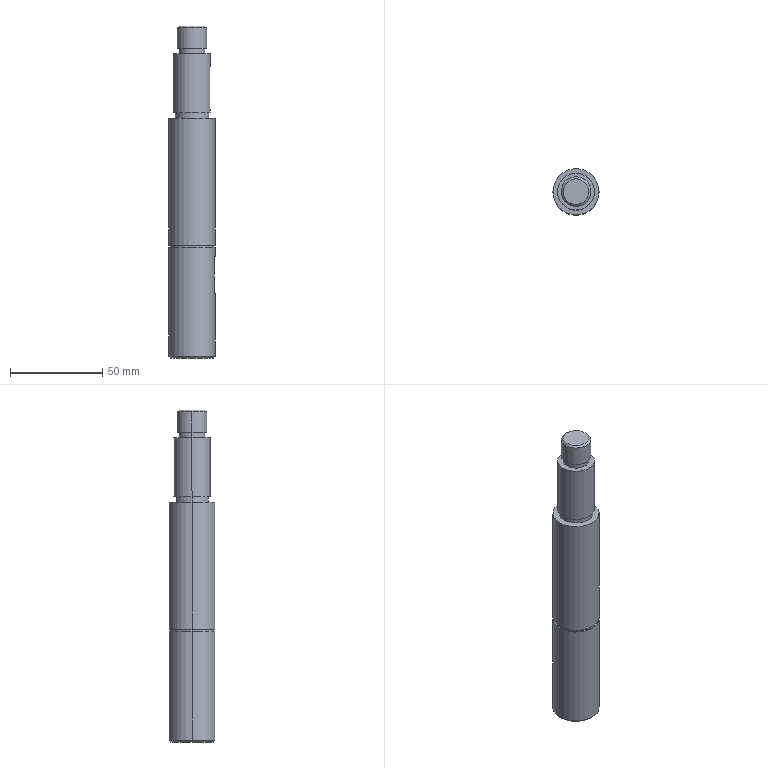Part | SolidWorks | features Chamfer 1, ICE 1, RefSurface 1, Revolution 1, ThickenCut 1 | 1 solid | 35 faces | box 25 x 25 x 180 mm | volume 76361 mm3 | cylinder 18 | plane 13 | cone 4 | commonest cylinder face diameters 25 x4 6 x3 14 x2 16 x2 18 x2 20 x2
STEP:
#1=CARTESIAN_POINT('',(-11.5,0.,0.));
#2=VERTEX_POINT('',#1);
#3=CARTESIAN_POINT('',(11.5,0.,0.));
#4=VERTEX_POINT('',#3);
#5=CARTESIAN_POINT('',(0.,0.,0.));
#6=DIRECTION('',(0.,0.,-1.));
#7=DIRECTION('',(-1.,0.,0.));
#8=AXIS2_PLACEMENT_3D('',#5,#6,#7);
#9=CIRCLE('',#8,11.5);
#10=EDGE_CURVE('',#2,#4,#9,.T.);
#11=ORIENTED_EDGE('',*,*,#10,.F.);
#12=CARTESIAN_POINT('',(-12.5,0.,1.));
#13=VERTEX_POINT('',#12);
#14=CARTESIAN_POINT('',(-11.5,0.,0.));
#15=DIRECTION('',(-0.7071,0.,0.7071));
#16=VECTOR('',#15,1000.);
#17=LINE('',#14,#16);
#18=EDGE_CURVE('',#2,#13,#17,.T.);
#19=ORIENTED_EDGE('',*,*,#18,.T.);
#20=CARTESIAN_POINT('',(12.5,0.,1.));
#21=VERTEX_POINT('',#20);
#22=CARTESIAN_POINT('',(0.,0.,1.));
#23=DIRECTION('',(0.,0.,1.));
#24=DIRECTION('',(-1.,0.,0.));
#25=AXIS2_PLACEMENT_3D('',#22,#23,#24);
#26=CIRCLE('',#25,12.5);
#27=EDGE_CURVE('',#21,#13,#26,.T.);
#28=ORIENTED_EDGE('',*,*,#27,.F.);
#29=CARTESIAN_POINT('',(11.5,0.,0.));
#30=DIRECTION('',(0.7071,0.,0.7071));
#31=VECTOR('',#30,1000.);
#32=LINE('',#29,#31);
#33=EDGE_CURVE('',#4,#21,#32,.T.);
#34=ORIENTED_EDGE('',*,*,#33,.F.);
#35=EDGE_LOOP('',(#11,#19,#28,#34));
#36=FACE_OUTER_BOUND('',#35,.T.);
#37=CARTESIAN_POINT('',(0.,0.,0.));
#38=DIRECTION('',(0.,0.,1.));
#39=DIRECTION('',(1.,0.,0.));
#40=AXIS2_PLACEMENT_3D('',#37,#38,#39);
#41=CONICAL_SURFACE('',#40,11.5,0.7854);
#42=ADVANCED_FACE('',(#36),#41,.T.);
#43=CARTESIAN_POINT('',(7.,0.,180.));
#44=VERTEX_POINT('',#43);
#45=CARTESIAN_POINT('',(-7.,0.,180.));
#46=VERTEX_POINT('',#45);
#47=CARTESIAN_POINT('',(0.,0.,180.));
#48=DIRECTION('',(0.,0.,1.));
#49=DIRECTION('',(1.,0.,0.));
#50=AXIS2_PLACEMENT_3D('',#47,#48,#49);
#51=CIRCLE('',#50,7.);
#52=EDGE_CURVE('',#44,#46,#51,.T.);
#53=ORIENTED_EDGE('',*,*,#52,.F.);
#54=CARTESIAN_POINT('',(8.,0.,179.));
#55=VERTEX_POINT('',#54);
#56=CARTESIAN_POINT('',(8.,0.,179.));
#57=DIRECTION('',(0.7071,0.,-0.7071));
#58=VECTOR('',#57,1000.);
#59=LINE('',#56,#58);
#60=EDGE_CURVE('',#44,#55,#59,.T.);
#61=ORIENTED_EDGE('',*,*,#60,.T.);
#62=CARTESIAN_POINT('',(-8.,0.,179.));
#63=VERTEX_POINT('',#62);
#64=CARTESIAN_POINT('',(0.,0.,179.));
#65=DIRECTION('',(0.,0.,-1.));
#66=DIRECTION('',(1.,0.,0.));
#67=AXIS2_PLACEMENT_3D('',#64,#65,#66);
#68=CIRCLE('',#67,8.);
#69=EDGE_CURVE('',#63,#55,#68,.T.);
#70=ORIENTED_EDGE('',*,*,#69,.F.);
#71=CARTESIAN_POINT('',(-8.,0.,179.));
#72=DIRECTION('',(-0.7071,0.,-0.7071));
#73=VECTOR('',#72,1000.);
#74=LINE('',#71,#73);
#75=EDGE_CURVE('',#46,#63,#74,.T.);
#76=ORIENTED_EDGE('',*,*,#75,.F.);
#77=EDGE_LOOP('',(#53,#61,#70,#76));
#78=FACE_OUTER_BOUND('',#77,.T.);
#79=CARTESIAN_POINT('',(0.,0.,179.));
#80=DIRECTION('',(0.,0.,-1.));
#81=DIRECTION('',(-1.,0.,0.));
#82=AXIS2_PLACEMENT_3D('',#79,#80,#81);
#83=CONICAL_SURFACE('',#82,8.,0.7854);
#84=ADVANCED_FACE('',(#78),#83,.T.);
#85=CARTESIAN_POINT('',(9.539,3.,156.));
#86=VERTEX_POINT('',#85);
#87=CARTESIAN_POINT('',(10.,0.,159.));
#88=VERTEX_POINT('',#87);
#89=CARTESIAN_POINT('',(9.539,3.,156.));
#90=CARTESIAN_POINT('',(9.539,3.,156.2));
#91=CARTESIAN_POINT('',(9.546,2.98,156.395));
#92=CARTESIAN_POINT('',(9.569,2.903,156.781));
#93=CARTESIAN_POINT('',(9.587,2.845,156.972));
#94=CARTESIAN_POINT('',(9.631,2.694,157.335));
#95=CARTESIAN_POINT('',(9.656,2.602,157.506));
#96=CARTESIAN_POINT('',(9.712,2.384,157.832));
#97=CARTESIAN_POINT('',(9.743,2.258,157.985));
#98=CARTESIAN_POINT('',(9.832,1.845,158.397));
#99=CARTESIAN_POINT('',(9.892,1.512,158.62));
#100=CARTESIAN_POINT('',(9.954,0.971,158.845));
#101=CARTESIAN_POINT('',(9.971,0.7806,158.903));
#102=CARTESIAN_POINT('',(9.994,0.3926,158.981));
#103=CARTESIAN_POINT('',(10.,0.197,159.));
#104=CARTESIAN_POINT('',(10.,0.,159.));
#105=B_SPLINE_CURVE_WITH_KNOTS('',3,(#89,#90,#91,#92,#93,#94,#95,#96,#97,#98,#99,#100,#101,#102,#103,#104),.UNSPECIFIED.,.F.,.F.,(4,2,2,2,2,2,2,4),(0.,0.0005898,0.00118,0.001769,0.002359,0.003539,0.004128,0.004718),.UNSPECIFIED.);
#106=EDGE_CURVE('',#86,#88,#105,.T.);
#107=ORIENTED_EDGE('',*,*,#106,.T.);
#108=CARTESIAN_POINT('',(6.5,0.,159.));
#109=VERTEX_POINT('',#108);
#110=CARTESIAN_POINT('',(12.5,0.,159.));
#111=DIRECTION('',(-1.,0.,0.));
#112=VECTOR('',#111,1000.);
#113=LINE('',#110,#112);
#114=EDGE_CURVE('',#88,#109,#113,.T.);
#115=ORIENTED_EDGE('',*,*,#114,.T.);
#116=CARTESIAN_POINT('',(6.5,3.,156.));
#117=VERTEX_POINT('',#116);
#118=CARTESIAN_POINT('',(6.5,0.,156.));
#119=DIRECTION('',(-1.,0.,0.));
#120=DIRECTION('',(0.,0.,1.));
#121=AXIS2_PLACEMENT_3D('',#118,#119,#120);
#122=CIRCLE('',#121,3.);
#123=EDGE_CURVE('',#109,#117,#122,.T.);
#124=ORIENTED_EDGE('',*,*,#123,.T.);
#125=CARTESIAN_POINT('',(12.5,3.,156.));
#126=DIRECTION('',(-1.,0.,0.));
#127=VECTOR('',#126,1000.);
#128=LINE('',#125,#127);
#129=EDGE_CURVE('',#86,#117,#128,.T.);
#130=ORIENTED_EDGE('',*,*,#129,.F.);
#131=EDGE_LOOP('',(#107,#115,#124,#130));
#132=FACE_OUTER_BOUND('',#131,.T.);
#133=CARTESIAN_POINT('',(12.5,0.,156.));
#134=DIRECTION('',(-1.,0.,0.));
#135=DIRECTION('',(0.,0.,1.));
#136=AXIS2_PLACEMENT_3D('',#133,#134,#135);
#137=CYLINDRICAL_SURFACE('',#136,3.);
#138=ADVANCED_FACE('',(#132),#137,.F.);
#139=CARTESIAN_POINT('',(-7.,0.,168.));
#140=VERTEX_POINT('',#139);
#141=CARTESIAN_POINT('',(7.,0.,168.));
#142=VERTEX_POINT('',#141);
#143=CARTESIAN_POINT('',(0.,0.,168.));
#144=DIRECTION('',(0.,0.,-1.));
#145=DIRECTION('',(-1.,0.,0.));
#146=AXIS2_PLACEMENT_3D('',#143,#144,#145);
#147=CIRCLE('',#146,7.);
#148=EDGE_CURVE('',#140,#142,#147,.T.);
#149=ORIENTED_EDGE('',*,*,#148,.T.);
#150=CARTESIAN_POINT('',(7.,0.,165.));
#151=VERTEX_POINT('',#150);
#152=CARTESIAN_POINT('',(7.,0.,180.));
#153=DIRECTION('',(0.,0.,-1.));
#154=VECTOR('',#153,1000.);
#155=LINE('',#152,#154);
#156=EDGE_CURVE('',#142,#151,#155,.T.);
#157=ORIENTED_EDGE('',*,*,#156,.T.);
#158=CARTESIAN_POINT('',(-7.,0.,165.));
#159=VERTEX_POINT('',#158);
#160=CARTESIAN_POINT('',(0.,0.,165.));
#161=DIRECTION('',(0.,0.,-1.));
#162=DIRECTION('',(-1.,0.,0.));
#163=AXIS2_PLACEMENT_3D('',#160,#161,#162);
#164=CIRCLE('',#163,7.);
#165=EDGE_CURVE('',#159,#151,#164,.T.);
#166=ORIENTED_EDGE('',*,*,#165,.F.);
#167=CARTESIAN_POINT('',(-7.,0.,180.));
#168=DIRECTION('',(0.,0.,-1.));
#169=VECTOR('',#168,1000.);
#170=LINE('',#167,#169);
#171=EDGE_CURVE('',#140,#159,#170,.T.);
#172=ORIENTED_EDGE('',*,*,#171,.F.);
#173=EDGE_LOOP('',(#149,#157,#166,#172));
#174=FACE_OUTER_BOUND('',#173,.T.);
#175=CARTESIAN_POINT('',(0.,0.,180.));
#176=DIRECTION('',(0.,0.,-1.));
#177=DIRECTION('',(-1.,0.,0.));
#178=AXIS2_PLACEMENT_3D('',#175,#176,#177);
#179=CYLINDRICAL_SURFACE('',#178,7.);
#180=ADVANCED_FACE('',(#174),#179,.T.);
#181=CARTESIAN_POINT('',(-10.,0.,165.));
#182=VERTEX_POINT('',#181);
#183=CARTESIAN_POINT('',(10.,0.,165.));
#184=VERTEX_POINT('',#183);
#185=CARTESIAN_POINT('',(0.,0.,165.));
#186=DIRECTION('',(0.,0.,-1.));
#187=DIRECTION('',(-1.,0.,0.));
#188=AXIS2_PLACEMENT_3D('',#185,#186,#187);
#189=CIRCLE('',#188,10.);
#190=EDGE_CURVE('',#182,#184,#189,.T.);
#191=ORIENTED_EDGE('',*,*,#190,.T.);
#192=CARTESIAN_POINT('',(10.,0.,180.));
#193=DIRECTION('',(0.,0.,-1.));
#194=VECTOR('',#193,1000.);
#195=LINE('',#192,#194);
#196=EDGE_CURVE('',#184,#88,#195,.T.);
#197=ORIENTED_EDGE('',*,*,#196,.T.);
#198=ORIENTED_EDGE('',*,*,#106,.F.);
#199=CARTESIAN_POINT('',(9.539,3.,137.));
#200=VERTEX_POINT('',#199);
#201=CARTESIAN_POINT('',(9.539,3.,180.));
#202=DIRECTION('',(0.,0.,1.));
#203=VECTOR('',#202,1000.);
#204=LINE('',#201,#203);
#205=EDGE_CURVE('',#200,#86,#204,.T.);
#206=ORIENTED_EDGE('',*,*,#205,.F.);
#207=CARTESIAN_POINT('',(10.,0.,134.));
#208=VERTEX_POINT('',#207);
#209=CARTESIAN_POINT('',(10.,0.,134.));
#210=CARTESIAN_POINT('',(10.,0.1968,134.));
#211=CARTESIAN_POINT('',(9.994,0.3967,134.02));
#212=CARTESIAN_POINT('',(9.971,0.7821,134.097));
#213=CARTESIAN_POINT('',(9.955,0.9695,134.154));
#214=CARTESIAN_POINT('',(9.912,1.334,134.306));
#215=CARTESIAN_POINT('',(9.887,1.507,134.399));
#216=CARTESIAN_POINT('',(9.832,1.831,134.616));
#217=CARTESIAN_POINT('',(9.802,1.983,134.741));
#218=CARTESIAN_POINT('',(9.742,2.26,135.017));
#219=CARTESIAN_POINT('',(9.713,2.383,135.167));
#220=CARTESIAN_POINT('',(9.657,2.6,135.491));
#221=CARTESIAN_POINT('',(9.63,2.694,135.667));
#222=CARTESIAN_POINT('',(9.587,2.845,136.028));
#223=CARTESIAN_POINT('',(9.57,2.902,136.215));
#224=CARTESIAN_POINT('',(9.546,2.98,136.601));
#225=CARTESIAN_POINT('',(9.539,3.,136.801));
#226=CARTESIAN_POINT('',(9.539,3.,137.));
#227=B_SPLINE_CURVE_WITH_KNOTS('',3,(#209,#210,#211,#212,#213,#214,#215,#216,#217,#218,#219,#220,#221,#222,#223,#224,#225,#226),.UNSPECIFIED.,.F.,.F.,(4,2,2,2,2,2,2,2,4),(0.004718,0.005307,0.005896,0.006485,0.007074,0.007663,0.008252,0.008842,0.009431),.UNSPECIFIED.);
#228=EDGE_CURVE('',#208,#200,#227,.T.);
#229=ORIENTED_EDGE('',*,*,#228,.F.);
#230=CARTESIAN_POINT('',(10.,0.,133.));
#231=VERTEX_POINT('',#230);
#232=CARTESIAN_POINT('',(10.,0.,180.));
#233=DIRECTION('',(0.,0.,-1.));
#234=VECTOR('',#233,1000.);
#235=LINE('',#232,#234);
#236=EDGE_CURVE('',#208,#231,#235,.T.);
#237=ORIENTED_EDGE('',*,*,#236,.T.);
#238=CARTESIAN_POINT('',(-10.,0.,133.));
#239=VERTEX_POINT('',#238);
#240=CARTESIAN_POINT('',(0.,0.,133.));
#241=DIRECTION('',(0.,0.,-1.));
#242=DIRECTION('',(-1.,0.,0.));
#243=AXIS2_PLACEMENT_3D('',#240,#241,#242);
#244=CIRCLE('',#243,10.);
#245=EDGE_CURVE('',#239,#231,#244,.T.);
#246=ORIENTED_EDGE('',*,*,#245,.F.);
#247=CARTESIAN_POINT('',(-10.,0.,180.));
#248=DIRECTION('',(0.,0.,-1.));
#249=VECTOR('',#248,1000.);
#250=LINE('',#247,#249);
#251=EDGE_CURVE('',#182,#239,#250,.T.);
#252=ORIENTED_EDGE('',*,*,#251,.F.);
#253=EDGE_LOOP('',(#191,#197,#198,#206,#229,#237,#246,#252));
#254=FACE_OUTER_BOUND('',#253,.T.);
#255=CARTESIAN_POINT('',(0.,0.,180.));
#256=DIRECTION('',(0.,0.,-1.));
#257=DIRECTION('',(-1.,0.,0.));
#258=AXIS2_PLACEMENT_3D('',#255,#256,#257);
#259=CYLINDRICAL_SURFACE('',#258,10.);
#260=ADVANCED_FACE('',(#254),#259,.T.);
#261=CARTESIAN_POINT('',(-9.,0.,133.));
#262=VERTEX_POINT('',#261);
#263=CARTESIAN_POINT('',(9.,0.,133.));
#264=VERTEX_POINT('',#263);
#265=CARTESIAN_POINT('',(0.,0.,133.));
#266=DIRECTION('',(0.,0.,-1.));
#267=DIRECTION('',(-1.,0.,0.));
#268=AXIS2_PLACEMENT_3D('',#265,#266,#267);
#269=CIRCLE('',#268,9.);
#270=EDGE_CURVE('',#262,#264,#269,.T.);
#271=ORIENTED_EDGE('',*,*,#270,.T.);
#272=CARTESIAN_POINT('',(9.,0.,130.));
#273=VERTEX_POINT('',#272);
#274=CARTESIAN_POINT('',(9.,0.,180.));
#275=DIRECTION('',(0.,0.,-1.));
#276=VECTOR('',#275,1000.);
#277=LINE('',#274,#276);
#278=EDGE_CURVE('',#264,#273,#277,.T.);
#279=ORIENTED_EDGE('',*,*,#278,.T.);
#280=CARTESIAN_POINT('',(-9.,0.,130.));
#281=VERTEX_POINT('',#280);
#282=CARTESIAN_POINT('',(0.,0.,130.));
#283=DIRECTION('',(0.,0.,-1.));
#284=DIRECTION('',(-1.,0.,0.));
#285=AXIS2_PLACEMENT_3D('',#282,#283,#284);
#286=CIRCLE('',#285,9.);
#287=EDGE_CURVE('',#281,#273,#286,.T.);
#288=ORIENTED_EDGE('',*,*,#287,.F.);
#289=CARTESIAN_POINT('',(-9.,0.,180.));
#290=DIRECTION('',(0.,0.,-1.));
#291=VECTOR('',#290,1000.);
#292=LINE('',#289,#291);
#293=EDGE_CURVE('',#262,#281,#292,.T.);
#294=ORIENTED_EDGE('',*,*,#293,.F.);
#295=EDGE_LOOP('',(#271,#279,#288,#294));
#296=FACE_OUTER_BOUND('',#295,.T.);
#297=CARTESIAN_POINT('',(0.,0.,180.));
#298=DIRECTION('',(0.,0.,-1.));
#299=DIRECTION('',(-1.,0.,0.));
#300=AXIS2_PLACEMENT_3D('',#297,#298,#299);
#301=CYLINDRICAL_SURFACE('',#300,9.);
#302=ADVANCED_FACE('',(#296),#301,.T.);
#303=CARTESIAN_POINT('',(-12.5,0.,130.));
#304=VERTEX_POINT('',#303);
#305=CARTESIAN_POINT('',(12.5,0.,130.));
#306=VERTEX_POINT('',#305);
#307=CARTESIAN_POINT('',(0.,0.,130.));
#308=DIRECTION('',(0.,0.,-1.));
#309=DIRECTION('',(-1.,0.,0.));
#310=AXIS2_PLACEMENT_3D('',#307,#308,#309);
#311=CIRCLE('',#310,12.5);
#312=EDGE_CURVE('',#304,#306,#311,.T.);
#313=ORIENTED_EDGE('',*,*,#312,.T.);
#314=CARTESIAN_POINT('',(12.5,0.,61.2));
#315=VERTEX_POINT('',#314);
#316=CARTESIAN_POINT('',(12.5,0.,180.));
#317=DIRECTION('',(0.,0.,-1.));
#318=VECTOR('',#317,1000.);
#319=LINE('',#316,#318);
#320=EDGE_CURVE('',#306,#315,#319,.T.);
#321=ORIENTED_EDGE('',*,*,#320,.T.);
#322=CARTESIAN_POINT('',(-12.5,0.,61.2));
#323=VERTEX_POINT('',#322);
#324=CARTESIAN_POINT('',(0.,0.,61.2));
#325=DIRECTION('',(0.,0.,-1.));
#326=DIRECTION('',(-1.,0.,0.));
#327=AXIS2_PLACEMENT_3D('',#324,#325,#326);
#328=CIRCLE('',#327,12.5);
#329=EDGE_CURVE('',#323,#315,#328,.T.);
#330=ORIENTED_EDGE('',*,*,#329,.F.);
#331=CARTESIAN_POINT('',(-12.5,0.,180.));
#332=DIRECTION('',(0.,0.,-1.));
#333=VECTOR('',#332,1000.);
#334=LINE('',#331,#333);
#335=EDGE_CURVE('',#304,#323,#334,.T.);
#336=ORIENTED_EDGE('',*,*,#335,.F.);
#337=EDGE_LOOP('',(#313,#321,#330,#336));
#338=FACE_OUTER_BOUND('',#337,.T.);
#339=CARTESIAN_POINT('',(0.,0.,180.));
#340=DIRECTION('',(0.,0.,-1.));
#341=DIRECTION('',(-1.,0.,0.));
#342=AXIS2_PLACEMENT_3D('',#339,#340,#341);
#343=CYLINDRICAL_SURFACE('',#342,12.5);
#344=ADVANCED_FACE('',(#338),#343,.T.);
#345=CARTESIAN_POINT('',(-11.9,0.,61.2));
#346=VERTEX_POINT('',#345);
#347=CARTESIAN_POINT('',(11.9,0.,61.2));
#348=VERTEX_POINT('',#347);
#349=CARTESIAN_POINT('',(0.,0.,61.2));
#350=DIRECTION('',(0.,0.,-1.));
#351=DIRECTION('',(-1.,0.,0.));
#352=AXIS2_PLACEMENT_3D('',#349,#350,#351);
#353=CIRCLE('',#352,11.9);
#354=EDGE_CURVE('',#346,#348,#353,.T.);
#355=ORIENTED_EDGE('',*,*,#354,.T.);
#356=CARTESIAN_POINT('',(11.9,0.,60.));
#357=VERTEX_POINT('',#356);
#358=CARTESIAN_POINT('',(11.9,0.,180.));
#359=DIRECTION('',(0.,0.,-1.));
#360=VECTOR('',#359,1000.);
#361=LINE('',#358,#360);
#362=EDGE_CURVE('',#348,#357,#361,.T.);
#363=ORIENTED_EDGE('',*,*,#362,.T.);
#364=CARTESIAN_POINT('',(-11.9,0.,60.));
#365=VERTEX_POINT('',#364);
#366=CARTESIAN_POINT('',(0.,0.,60.));
#367=DIRECTION('',(0.,0.,-1.));
#368=DIRECTION('',(-1.,0.,0.));
#369=AXIS2_PLACEMENT_3D('',#366,#367,#368);
#370=CIRCLE('',#369,11.9);
#371=EDGE_CURVE('',#365,#357,#370,.T.);
#372=ORIENTED_EDGE('',*,*,#371,.F.);
#373=CARTESIAN_POINT('',(-11.9,0.,180.));
#374=DIRECTION('',(0.,0.,-1.));
#375=VECTOR('',#374,1000.);
#376=LINE('',#373,#375);
#377=EDGE_CURVE('',#346,#365,#376,.T.);
#378=ORIENTED_EDGE('',*,*,#377,.F.);
#379=EDGE_LOOP('',(#355,#363,#372,#378));
#380=FACE_OUTER_BOUND('',#379,.T.);
#381=CARTESIAN_POINT('',(0.,0.,180.));
#382=DIRECTION('',(0.,0.,-1.));
#383=DIRECTION('',(-1.,0.,0.));
#384=AXIS2_PLACEMENT_3D('',#381,#382,#383);
#385=CYLINDRICAL_SURFACE('',#384,11.9);
#386=ADVANCED_FACE('',(#380),#385,.T.);
#387=CARTESIAN_POINT('',(-12.5,0.,60.));
#388=VERTEX_POINT('',#387);
#389=CARTESIAN_POINT('',(12.5,0.,60.));
#390=VERTEX_POINT('',#389);
#391=CARTESIAN_POINT('',(0.,0.,60.));
#392=DIRECTION('',(0.,0.,-1.));
#393=DIRECTION('',(-1.,0.,0.));
#394=AXIS2_PLACEMENT_3D('',#391,#392,#393);
#395=CIRCLE('',#394,12.5);
#396=EDGE_CURVE('',#388,#390,#395,.T.);
#397=ORIENTED_EDGE('',*,*,#396,.T.);
#398=CARTESIAN_POINT('',(12.5,0.,55.037));
#399=VERTEX_POINT('',#398);
#400=CARTESIAN_POINT('',(12.5,0.,180.));
#401=DIRECTION('',(0.,0.,-1.));
#402=VECTOR('',#401,1000.);
#403=LINE('',#400,#402);
#404=EDGE_CURVE('',#390,#399,#403,.T.);
#405=ORIENTED_EDGE('',*,*,#404,.T.);
#406=CARTESIAN_POINT('',(12.135,3.,54.866));
#407=VERTEX_POINT('',#406);
#408=CARTESIAN_POINT('',(12.5,0.,55.037));
#409=CARTESIAN_POINT('',(12.5,1.018,55.037));
#410=CARTESIAN_POINT('',(12.377,2.018,54.985));
#411=CARTESIAN_POINT('',(12.135,3.,54.866));
#412=B_SPLINE_CURVE_WITH_KNOTS('',3,(#408,#409,#410,#411),.UNSPECIFIED.,.F.,.F.,(4,4),(0.,0.003027),.UNSPECIFIED.);
#413=EDGE_CURVE('',#399,#407,#412,.T.);
#414=ORIENTED_EDGE('',*,*,#413,.T.);
#415=CARTESIAN_POINT('',(12.135,3.,35.134));
#416=VERTEX_POINT('',#415);
#417=CARTESIAN_POINT('',(12.135,3.,130.));
#418=DIRECTION('',(0.,0.,-1.));
#419=VECTOR('',#418,1000.);
#420=LINE('',#417,#419);
#421=EDGE_CURVE('',#407,#416,#420,.T.);
#422=ORIENTED_EDGE('',*,*,#421,.T.);
#423=CARTESIAN_POINT('',(12.5,0.,34.963));
#424=VERTEX_POINT('',#423);
#425=CARTESIAN_POINT('',(12.135,3.,35.134));
#426=CARTESIAN_POINT('',(12.377,2.018,35.015));
#427=CARTESIAN_POINT('',(12.5,1.018,34.963));
#428=CARTESIAN_POINT('',(12.5,0.,34.963));
#429=B_SPLINE_CURVE_WITH_KNOTS('',3,(#425,#426,#427,#428),.UNSPECIFIED.,.F.,.F.,(4,4),(0.,0.003027),.UNSPECIFIED.);
#430=EDGE_CURVE('',#416,#424,#429,.T.);
#431=ORIENTED_EDGE('',*,*,#430,.T.);
#432=CARTESIAN_POINT('',(12.5,0.,180.));
#433=DIRECTION('',(0.,0.,-1.));
#434=VECTOR('',#433,1000.);
#435=LINE('',#432,#434);
#436=EDGE_CURVE('',#424,#21,#435,.T.);
#437=ORIENTED_EDGE('',*,*,#436,.T.);
#438=ORIENTED_EDGE('',*,*,#27,.T.);
#439=CARTESIAN_POINT('',(-12.5,0.,180.));
#440=DIRECTION('',(0.,0.,-1.));
#441=VECTOR('',#440,1000.);
#442=LINE('',#439,#441);
#443=EDGE_CURVE('',#388,#13,#442,.T.);
#444=ORIENTED_EDGE('',*,*,#443,.F.);
#445=EDGE_LOOP('',(#397,#405,#414,#422,#431,#437,#438,#444));
#446=FACE_OUTER_BOUND('',#445,.T.);
#447=CARTESIAN_POINT('',(0.,0.,180.));
#448=DIRECTION('',(0.,0.,-1.));
#449=DIRECTION('',(-1.,0.,0.));
#450=AXIS2_PLACEMENT_3D('',#447,#448,#449);
#451=CYLINDRICAL_SURFACE('',#450,12.5);
#452=ADVANCED_FACE('',(#446),#451,.T.);
#453=ORIENTED_EDGE('',*,*,#69,.T.);
#454=CARTESIAN_POINT('',(8.,0.,168.));
#455=VERTEX_POINT('',#454);
#456=CARTESIAN_POINT('',(8.,0.,180.));
#457=DIRECTION('',(0.,0.,-1.));
#458=VECTOR('',#457,1000.);
#459=LINE('',#456,#458);
#460=EDGE_CURVE('',#55,#455,#459,.T.);
#461=ORIENTED_EDGE('',*,*,#460,.T.);
#462=CARTESIAN_POINT('',(-8.,0.,168.));
#463=VERTEX_POINT('',#462);
#464=CARTESIAN_POINT('',(0.,0.,168.));
#465=DIRECTION('',(0.,0.,-1.));
#466=DIRECTION('',(-1.,0.,0.));
#467=AXIS2_PLACEMENT_3D('',#464,#465,#466);
#468=CIRCLE('',#467,8.);
#469=EDGE_CURVE('',#463,#455,#468,.T.);
#470=ORIENTED_EDGE('',*,*,#469,.F.);
#471=CARTESIAN_POINT('',(-8.,0.,180.));
#472=DIRECTION('',(0.,0.,-1.));
#473=VECTOR('',#472,1000.);
#474=LINE('',#471,#473);
#475=EDGE_CURVE('',#63,#463,#474,.T.);
#476=ORIENTED_EDGE('',*,*,#475,.F.);
#477=EDGE_LOOP('',(#453,#461,#470,#476));
#478=FACE_OUTER_BOUND('',#477,.T.);
#479=CARTESIAN_POINT('',(0.,0.,180.));
#480=DIRECTION('',(0.,0.,-1.));
#481=DIRECTION('',(-1.,0.,0.));
#482=AXIS2_PLACEMENT_3D('',#479,#480,#481);
#483=CYLINDRICAL_SURFACE('',#482,8.);
#484=ADVANCED_FACE('',(#478),#483,.T.);
#485=ORIENTED_EDGE('',*,*,#460,.F.);
#486=CARTESIAN_POINT('',(0.,0.,179.));
#487=DIRECTION('',(0.,0.,-1.));
#488=DIRECTION('',(1.,0.,0.));
#489=AXIS2_PLACEMENT_3D('',#486,#487,#488);
#490=CIRCLE('',#489,8.);
#491=EDGE_CURVE('',#55,#63,#490,.T.);
#492=ORIENTED_EDGE('',*,*,#491,.T.);
#493=ORIENTED_EDGE('',*,*,#475,.T.);
#494=CARTESIAN_POINT('',(0.,0.,168.));
#495=DIRECTION('',(0.,0.,-1.));
#496=DIRECTION('',(-1.,0.,0.));
#497=AXIS2_PLACEMENT_3D('',#494,#495,#496);
#498=CIRCLE('',#497,8.);
#499=EDGE_CURVE('',#455,#463,#498,.T.);
#500=ORIENTED_EDGE('',*,*,#499,.F.);
#501=EDGE_LOOP('',(#485,#492,#493,#500));
#502=FACE_OUTER_BOUND('',#501,.T.);
#503=CARTESIAN_POINT('',(0.,0.,180.));
#504=DIRECTION('',(0.,0.,-1.));
#505=DIRECTION('',(-1.,0.,0.));
#506=AXIS2_PLACEMENT_3D('',#503,#504,#505);
#507=CYLINDRICAL_SURFACE('',#506,8.);
#508=ADVANCED_FACE('',(#502),#507,.T.);
#509=CARTESIAN_POINT('',(0.,0.,180.));
#510=DIRECTION('',(0.,0.,1.));
#511=DIRECTION('',(1.,0.,0.));
#512=AXIS2_PLACEMENT_3D('',#509,#510,#511);
#513=CIRCLE('',#512,7.);
#514=EDGE_CURVE('',#46,#44,#513,.T.);
#515=ORIENTED_EDGE('',*,*,#514,.T.);
#516=ORIENTED_EDGE('',*,*,#52,.T.);
#517=EDGE_LOOP('',(#515,#516));
#518=FACE_OUTER_BOUND('',#517,.T.);
#519=CARTESIAN_POINT('',(8.,0.,180.));
#520=DIRECTION('',(0.,0.,1.));
#521=DIRECTION('',(1.,0.,0.));
#522=AXIS2_PLACEMENT_3D('',#519,#520,#521);
#523=PLANE('',#522);
#524=ADVANCED_FACE('',(#518),#523,.T.);
#525=CARTESIAN_POINT('',(0.,0.,0.));
#526=DIRECTION('',(0.,0.,-1.));
#527=DIRECTION('',(-1.,0.,0.));
#528=AXIS2_PLACEMENT_3D('',#525,#526,#527);
#529=CIRCLE('',#528,11.5);
#530=EDGE_CURVE('',#4,#2,#529,.T.);
#531=ORIENTED_EDGE('',*,*,#530,.T.);
#532=ORIENTED_EDGE('',*,*,#10,.T.);
#533=EDGE_LOOP('',(#531,#532));
#534=FACE_OUTER_BOUND('',#533,.T.);
#535=CARTESIAN_POINT('',(0.,0.,0.));
#536=DIRECTION('',(0.,0.,-1.));
#537=DIRECTION('',(-1.,0.,0.));
#538=AXIS2_PLACEMENT_3D('',#535,#536,#537);
#539=PLANE('',#538);
#540=ADVANCED_FACE('',(#534),#539,.T.);
#541=ORIENTED_EDGE('',*,*,#404,.F.);
#542=CARTESIAN_POINT('',(0.,0.,60.));
#543=DIRECTION('',(0.,0.,-1.));
#544=DIRECTION('',(-1.,0.,0.));
#545=AXIS2_PLACEMENT_3D('',#542,#543,#544);
#546=CIRCLE('',#545,12.5);
#547=EDGE_CURVE('',#390,#388,#546,.T.);
#548=ORIENTED_EDGE('',*,*,#547,.T.);
#549=ORIENTED_EDGE('',*,*,#443,.T.);
#550=CARTESIAN_POINT('',(0.,0.,1.));
#551=DIRECTION('',(0.,0.,1.));
#552=DIRECTION('',(-1.,0.,0.));
#553=AXIS2_PLACEMENT_3D('',#550,#551,#552);
#554=CIRCLE('',#553,12.5);
#555=EDGE_CURVE('',#13,#21,#554,.T.);
#556=ORIENTED_EDGE('',*,*,#555,.T.);
#557=ORIENTED_EDGE('',*,*,#436,.F.);
#558=CARTESIAN_POINT('',(12.135,-3.,35.134));
#559=VERTEX_POINT('',#558);
#560=CARTESIAN_POINT('',(12.5,0.,34.963));
#561=CARTESIAN_POINT('',(12.5,-1.018,34.963));
#562=CARTESIAN_POINT('',(12.377,-2.018,35.015));
#563=CARTESIAN_POINT('',(12.135,-3.,35.134));
#564=B_SPLINE_CURVE_WITH_KNOTS('',3,(#560,#561,#562,#563),.UNSPECIFIED.,.F.,.F.,(4,4),(0.003027,0.006054),.UNSPECIFIED.);
#565=EDGE_CURVE('',#424,#559,#564,.T.);
#566=ORIENTED_EDGE('',*,*,#565,.T.);
#567=CARTESIAN_POINT('',(12.135,-3.,54.866));
#568=VERTEX_POINT('',#567);
#569=CARTESIAN_POINT('',(12.135,-3.,130.));
#570=DIRECTION('',(0.,0.,-1.));
#571=VECTOR('',#570,1000.);
#572=LINE('',#569,#571);
#573=EDGE_CURVE('',#568,#559,#572,.T.);
#574=ORIENTED_EDGE('',*,*,#573,.F.);
#575=CARTESIAN_POINT('',(12.135,-3.,54.866));
#576=CARTESIAN_POINT('',(12.377,-2.018,54.985));
#577=CARTESIAN_POINT('',(12.5,-1.018,55.037));
#578=CARTESIAN_POINT('',(12.5,0.,55.037));
#579=B_SPLINE_CURVE_WITH_KNOTS('',3,(#575,#576,#577,#578),.UNSPECIFIED.,.F.,.F.,(4,4),(-0.003027,0.),.UNSPECIFIED.);
#580=EDGE_CURVE('',#568,#399,#579,.T.);
#581=ORIENTED_EDGE('',*,*,#580,.T.);
#582=EDGE_LOOP('',(#541,#548,#549,#556,#557,#566,#574,#581));
#583=FACE_OUTER_BOUND('',#582,.T.);
#584=CARTESIAN_POINT('',(0.,0.,180.));
#585=DIRECTION('',(0.,0.,-1.));
#586=DIRECTION('',(-1.,0.,0.));
#587=AXIS2_PLACEMENT_3D('',#584,#585,#586);
#588=CYLINDRICAL_SURFACE('',#587,12.5);
#589=ADVANCED_FACE('',(#583),#588,.T.);
#590=ORIENTED_EDGE('',*,*,#371,.T.);
#591=CARTESIAN_POINT('',(0.,0.,60.));
#592=DIRECTION('',(0.,0.,-1.));
#593=DIRECTION('',(-1.,0.,0.));
#594=AXIS2_PLACEMENT_3D('',#591,#592,#593);
#595=CIRCLE('',#594,11.9);
#596=EDGE_CURVE('',#357,#365,#595,.T.);
#597=ORIENTED_EDGE('',*,*,#596,.T.);
#598=EDGE_LOOP('',(#590,#597));
#599=FACE_BOUND('',#598,.T.);
#600=ORIENTED_EDGE('',*,*,#396,.F.);
#601=ORIENTED_EDGE('',*,*,#547,.F.);
#602=EDGE_LOOP('',(#600,#601));
#603=FACE_OUTER_BOUND('',#602,.T.);
#604=CARTESIAN_POINT('',(12.5,0.,60.));
#605=DIRECTION('',(0.,0.,1.));
#606=DIRECTION('',(1.,0.,0.));
#607=AXIS2_PLACEMENT_3D('',#604,#605,#606);
#608=PLANE('',#607);
#609=ADVANCED_FACE('',(#599,#603),#608,.T.);
#610=ORIENTED_EDGE('',*,*,#362,.F.);
#611=CARTESIAN_POINT('',(0.,0.,61.2));
#612=DIRECTION('',(0.,0.,-1.));
#613=DIRECTION('',(-1.,0.,0.));
#614=AXIS2_PLACEMENT_3D('',#611,#612,#613);
#615=CIRCLE('',#614,11.9);
#616=EDGE_CURVE('',#348,#346,#615,.T.);
#617=ORIENTED_EDGE('',*,*,#616,.T.);
#618=ORIENTED_EDGE('',*,*,#377,.T.);
#619=ORIENTED_EDGE('',*,*,#596,.F.);
#620=EDGE_LOOP('',(#610,#617,#618,#619));
#621=FACE_OUTER_BOUND('',#620,.T.);
#622=CARTESIAN_POINT('',(0.,0.,180.));
#623=DIRECTION('',(0.,0.,-1.));
#624=DIRECTION('',(-1.,0.,0.));
#625=AXIS2_PLACEMENT_3D('',#622,#623,#624);
#626=CYLINDRICAL_SURFACE('',#625,11.9);
#627=ADVANCED_FACE('',(#621),#626,.T.);
#628=ORIENTED_EDGE('',*,*,#329,.T.);
#629=CARTESIAN_POINT('',(0.,0.,61.2));
#630=DIRECTION('',(0.,0.,-1.));
#631=DIRECTION('',(-1.,0.,0.));
#632=AXIS2_PLACEMENT_3D('',#629,#630,#631);
#633=CIRCLE('',#632,12.5);
#634=EDGE_CURVE('',#315,#323,#633,.T.);
#635=ORIENTED_EDGE('',*,*,#634,.T.);
#636=EDGE_LOOP('',(#628,#635));
#637=FACE_OUTER_BOUND('',#636,.T.);
#638=ORIENTED_EDGE('',*,*,#354,.F.);
#639=ORIENTED_EDGE('',*,*,#616,.F.);
#640=EDGE_LOOP('',(#638,#639));
#641=FACE_BOUND('',#640,.T.);
#642=CARTESIAN_POINT('',(11.9,0.,61.2));
#643=DIRECTION('',(0.,0.,-1.));
#644=DIRECTION('',(-1.,0.,0.));
#645=AXIS2_PLACEMENT_3D('',#642,#643,#644);
#646=PLANE('',#645);
#647=ADVANCED_FACE('',(#637,#641),#646,.T.);
#648=ORIENTED_EDGE('',*,*,#320,.F.);
#649=CARTESIAN_POINT('',(0.,0.,130.));
#650=DIRECTION('',(0.,0.,-1.));
#651=DIRECTION('',(-1.,0.,0.));
#652=AXIS2_PLACEMENT_3D('',#649,#650,#651);
#653=CIRCLE('',#652,12.5);
#654=EDGE_CURVE('',#306,#304,#653,.T.);
#655=ORIENTED_EDGE('',*,*,#654,.T.);
#656=ORIENTED_EDGE('',*,*,#335,.T.);
#657=ORIENTED_EDGE('',*,*,#634,.F.);
#658=EDGE_LOOP('',(#648,#655,#656,#657));
#659=FACE_OUTER_BOUND('',#658,.T.);
#660=CARTESIAN_POINT('',(0.,0.,180.));
#661=DIRECTION('',(0.,0.,-1.));
#662=DIRECTION('',(-1.,0.,0.));
#663=AXIS2_PLACEMENT_3D('',#660,#661,#662);
#664=CYLINDRICAL_SURFACE('',#663,12.5);
#665=ADVANCED_FACE('',(#659),#664,.T.);
#666=ORIENTED_EDGE('',*,*,#287,.T.);
#667=CARTESIAN_POINT('',(0.,0.,130.));
#668=DIRECTION('',(0.,0.,-1.));
#669=DIRECTION('',(-1.,0.,0.));
#670=AXIS2_PLACEMENT_3D('',#667,#668,#669);
#671=CIRCLE('',#670,9.);
#672=EDGE_CURVE('',#273,#281,#671,.T.);
#673=ORIENTED_EDGE('',*,*,#672,.T.);
#674=EDGE_LOOP('',(#666,#673));
#675=FACE_BOUND('',#674,.T.);
#676=ORIENTED_EDGE('',*,*,#312,.F.);
#677=ORIENTED_EDGE('',*,*,#654,.F.);
#678=EDGE_LOOP('',(#676,#677));
#679=FACE_OUTER_BOUND('',#678,.T.);
#680=CARTESIAN_POINT('',(12.5,0.,130.));
#681=DIRECTION('',(0.,0.,1.));
#682=DIRECTION('',(1.,0.,0.));
#683=AXIS2_PLACEMENT_3D('',#680,#681,#682);
#684=PLANE('',#683);
#685=ADVANCED_FACE('',(#675,#679),#684,.T.);
#686=ORIENTED_EDGE('',*,*,#278,.F.);
#687=CARTESIAN_POINT('',(0.,0.,133.));
#688=DIRECTION('',(0.,0.,-1.));
#689=DIRECTION('',(-1.,0.,0.));
#690=AXIS2_PLACEMENT_3D('',#687,#688,#689);
#691=CIRCLE('',#690,9.);
#692=EDGE_CURVE('',#264,#262,#691,.T.);
#693=ORIENTED_EDGE('',*,*,#692,.T.);
#694=ORIENTED_EDGE('',*,*,#293,.T.);
#695=ORIENTED_EDGE('',*,*,#672,.F.);
#696=EDGE_LOOP('',(#686,#693,#694,#695));
#697=FACE_OUTER_BOUND('',#696,.T.);
#698=CARTESIAN_POINT('',(0.,0.,180.));
#699=DIRECTION('',(0.,0.,-1.));
#700=DIRECTION('',(-1.,0.,0.));
#701=AXIS2_PLACEMENT_3D('',#698,#699,#700);
#702=CYLINDRICAL_SURFACE('',#701,9.);
#703=ADVANCED_FACE('',(#697),#702,.T.);
#704=ORIENTED_EDGE('',*,*,#245,.T.);
#705=CARTESIAN_POINT('',(0.,0.,133.));
#706=DIRECTION('',(0.,0.,-1.));
#707=DIRECTION('',(-1.,0.,0.));
#708=AXIS2_PLACEMENT_3D('',#705,#706,#707);
#709=CIRCLE('',#708,10.);
#710=EDGE_CURVE('',#231,#239,#709,.T.);
#711=ORIENTED_EDGE('',*,*,#710,.T.);
#712=EDGE_LOOP('',(#704,#711));
#713=FACE_OUTER_BOUND('',#712,.T.);
#714=ORIENTED_EDGE('',*,*,#270,.F.);
#715=ORIENTED_EDGE('',*,*,#692,.F.);
#716=EDGE_LOOP('',(#714,#715));
#717=FACE_BOUND('',#716,.T.);
#718=CARTESIAN_POINT('',(9.,0.,133.));
#719=DIRECTION('',(0.,0.,-1.));
#720=DIRECTION('',(-1.,0.,0.));
#721=AXIS2_PLACEMENT_3D('',#718,#719,#720);
#722=PLANE('',#721);
#723=ADVANCED_FACE('',(#713,#717),#722,.T.);
#724=ORIENTED_EDGE('',*,*,#196,.F.);
#725=CARTESIAN_POINT('',(0.,0.,165.));
#726=DIRECTION('',(0.,0.,-1.));
#727=DIRECTION('',(-1.,0.,0.));
#728=AXIS2_PLACEMENT_3D('',#725,#726,#727);
#729=CIRCLE('',#728,10.);
#730=EDGE_CURVE('',#184,#182,#729,.T.);
#731=ORIENTED_EDGE('',*,*,#730,.T.);
#732=ORIENTED_EDGE('',*,*,#251,.T.);
#733=ORIENTED_EDGE('',*,*,#710,.F.);
#734=ORIENTED_EDGE('',*,*,#236,.F.);
#735=CARTESIAN_POINT('',(9.539,-3.,137.));
#736=VERTEX_POINT('',#735);
#737=CARTESIAN_POINT('',(9.539,-3.,137.));
#738=CARTESIAN_POINT('',(9.539,-3.,136.8));
#739=CARTESIAN_POINT('',(9.546,-2.98,136.605));
#740=CARTESIAN_POINT('',(9.569,-2.903,136.219));
#741=CARTESIAN_POINT('',(9.587,-2.845,136.028));
#742=CARTESIAN_POINT('',(9.631,-2.694,135.665));
#743=CARTESIAN_POINT('',(9.656,-2.602,135.494));
#744=CARTESIAN_POINT('',(9.712,-2.384,135.168));
#745=CARTESIAN_POINT('',(9.743,-2.258,135.015));
#746=CARTESIAN_POINT('',(9.832,-1.845,134.603));
#747=CARTESIAN_POINT('',(9.892,-1.512,134.38));
#748=CARTESIAN_POINT('',(9.954,-0.971,134.155));
#749=CARTESIAN_POINT('',(9.971,-0.7806,134.097));
#750=CARTESIAN_POINT('',(9.994,-0.3926,134.019));
#751=CARTESIAN_POINT('',(10.,-0.197,134.));
#752=CARTESIAN_POINT('',(10.,0.,134.));
#753=B_SPLINE_CURVE_WITH_KNOTS('',3,(#737,#738,#739,#740,#741,#742,#743,#744,#745,#746,#747,#748,#749,#750,#751,#752),.UNSPECIFIED.,.F.,.F.,(4,2,2,2,2,2,2,4),(0.,0.0005898,0.00118,0.001769,0.002359,0.003539,0.004128,0.004718),.UNSPECIFIED.);
#754=EDGE_CURVE('',#736,#208,#753,.T.);
#755=ORIENTED_EDGE('',*,*,#754,.F.);
#756=CARTESIAN_POINT('',(9.539,-3.,156.));
#757=VERTEX_POINT('',#756);
#758=CARTESIAN_POINT('',(9.539,-3.,180.));
#759=DIRECTION('',(0.,0.,-1.));
#760=VECTOR('',#759,1000.);
#761=LINE('',#758,#760);
#762=EDGE_CURVE('',#757,#736,#761,.T.);
#763=ORIENTED_EDGE('',*,*,#762,.F.);
#764=CARTESIAN_POINT('',(10.,0.,159.));
#765=CARTESIAN_POINT('',(10.,-0.1968,159.));
#766=CARTESIAN_POINT('',(9.994,-0.3967,158.98));
#767=CARTESIAN_POINT('',(9.971,-0.7821,158.903));
#768=CARTESIAN_POINT('',(9.955,-0.9695,158.846));
#769=CARTESIAN_POINT('',(9.912,-1.334,158.694));
#770=CARTESIAN_POINT('',(9.887,-1.507,158.601));
#771=CARTESIAN_POINT('',(9.832,-1.831,158.384));
#772=CARTESIAN_POINT('',(9.802,-1.983,158.259));
#773=CARTESIAN_POINT('',(9.742,-2.26,157.983));
#774=CARTESIAN_POINT('',(9.713,-2.383,157.833));
#775=CARTESIAN_POINT('',(9.657,-2.6,157.509));
#776=CARTESIAN_POINT('',(9.63,-2.694,157.333));
#777=CARTESIAN_POINT('',(9.587,-2.845,156.972));
#778=CARTESIAN_POINT('',(9.57,-2.902,156.785));
#779=CARTESIAN_POINT('',(9.546,-2.98,156.399));
#780=CARTESIAN_POINT('',(9.539,-3.,156.199));
#781=CARTESIAN_POINT('',(9.539,-3.,156.));
#782=B_SPLINE_CURVE_WITH_KNOTS('',3,(#764,#765,#766,#767,#768,#769,#770,#771,#772,#773,#774,#775,#776,#777,#778,#779,#780,#781),.UNSPECIFIED.,.F.,.F.,(4,2,2,2,2,2,2,2,4),(0.004718,0.005307,0.005896,0.006485,0.007074,0.007663,0.008252,0.008842,0.009431),.UNSPECIFIED.);
#783=EDGE_CURVE('',#88,#757,#782,.T.);
#784=ORIENTED_EDGE('',*,*,#783,.F.);
#785=EDGE_LOOP('',(#724,#731,#732,#733,#734,#755,#763,#784));
#786=FACE_OUTER_BOUND('',#785,.T.);
#787=CARTESIAN_POINT('',(0.,0.,180.));
#788=DIRECTION('',(0.,0.,-1.));
#789=DIRECTION('',(-1.,0.,0.));
#790=AXIS2_PLACEMENT_3D('',#787,#788,#789);
#791=CYLINDRICAL_SURFACE('',#790,10.);
#792=ADVANCED_FACE('',(#786),#791,.T.);
#793=ORIENTED_EDGE('',*,*,#165,.T.);
#794=CARTESIAN_POINT('',(0.,0.,165.));
#795=DIRECTION('',(0.,0.,-1.));
#796=DIRECTION('',(-1.,0.,0.));
#797=AXIS2_PLACEMENT_3D('',#794,#795,#796);
#798=CIRCLE('',#797,7.);
#799=EDGE_CURVE('',#151,#159,#798,.T.);
#800=ORIENTED_EDGE('',*,*,#799,.T.);
#801=EDGE_LOOP('',(#793,#800));
#802=FACE_BOUND('',#801,.T.);
#803=ORIENTED_EDGE('',*,*,#190,.F.);
#804=ORIENTED_EDGE('',*,*,#730,.F.);
#805=EDGE_LOOP('',(#803,#804));
#806=FACE_OUTER_BOUND('',#805,.T.);
#807=CARTESIAN_POINT('',(10.,0.,165.));
#808=DIRECTION('',(0.,0.,1.));
#809=DIRECTION('',(1.,0.,0.));
#810=AXIS2_PLACEMENT_3D('',#807,#808,#809);
#811=PLANE('',#810);
#812=ADVANCED_FACE('',(#802,#806),#811,.T.);
#813=ORIENTED_EDGE('',*,*,#156,.F.);
#814=CARTESIAN_POINT('',(0.,0.,168.));
#815=DIRECTION('',(0.,0.,-1.));
#816=DIRECTION('',(-1.,0.,0.));
#817=AXIS2_PLACEMENT_3D('',#814,#815,#816);
#818=CIRCLE('',#817,7.);
#819=EDGE_CURVE('',#142,#140,#818,.T.);
#820=ORIENTED_EDGE('',*,*,#819,.T.);
#821=ORIENTED_EDGE('',*,*,#171,.T.);
#822=ORIENTED_EDGE('',*,*,#799,.F.);
#823=EDGE_LOOP('',(#813,#820,#821,#822));
#824=FACE_OUTER_BOUND('',#823,.T.);
#825=CARTESIAN_POINT('',(0.,0.,180.));
#826=DIRECTION('',(0.,0.,-1.));
#827=DIRECTION('',(-1.,0.,0.));
#828=AXIS2_PLACEMENT_3D('',#825,#826,#827);
#829=CYLINDRICAL_SURFACE('',#828,7.);
#830=ADVANCED_FACE('',(#824),#829,.T.);
#831=ORIENTED_EDGE('',*,*,#469,.T.);
#832=ORIENTED_EDGE('',*,*,#499,.T.);
#833=EDGE_LOOP('',(#831,#832));
#834=FACE_OUTER_BOUND('',#833,.T.);
#835=ORIENTED_EDGE('',*,*,#148,.F.);
#836=ORIENTED_EDGE('',*,*,#819,.F.);
#837=EDGE_LOOP('',(#835,#836));
#838=FACE_BOUND('',#837,.T.);
#839=CARTESIAN_POINT('',(7.,0.,168.));
#840=DIRECTION('',(0.,0.,-1.));
#841=DIRECTION('',(-1.,0.,0.));
#842=AXIS2_PLACEMENT_3D('',#839,#840,#841);
#843=PLANE('',#842);
#844=ADVANCED_FACE('',(#834,#838),#843,.T.);
#845=ORIENTED_EDGE('',*,*,#573,.T.);
#846=CARTESIAN_POINT('',(17.,-3.,45.));
#847=DIRECTION('',(0.,1.,0.));
#848=DIRECTION('',(0.,0.,1.));
#849=AXIS2_PLACEMENT_3D('',#846,#847,#848);
#850=CIRCLE('',#849,11.);
#851=EDGE_CURVE('',#559,#568,#850,.T.);
#852=ORIENTED_EDGE('',*,*,#851,.T.);
#853=EDGE_LOOP('',(#845,#852));
#854=FACE_OUTER_BOUND('',#853,.T.);
#855=CARTESIAN_POINT('',(17.,-3.,45.));
#856=DIRECTION('',(0.,1.,0.));
#857=DIRECTION('',(1.,0.,0.));
#858=AXIS2_PLACEMENT_3D('',#855,#856,#857);
#859=PLANE('',#858);
#860=ADVANCED_FACE('',(#854),#859,.T.);
#861=ORIENTED_EDGE('',*,*,#851,.F.);
#862=ORIENTED_EDGE('',*,*,#565,.F.);
#863=ORIENTED_EDGE('',*,*,#430,.F.);
#864=CARTESIAN_POINT('',(17.,3.,45.));
#865=DIRECTION('',(0.,1.,0.));
#866=DIRECTION('',(0.,0.,1.));
#867=AXIS2_PLACEMENT_3D('',#864,#865,#866);
#868=CIRCLE('',#867,11.);
#869=EDGE_CURVE('',#416,#407,#868,.T.);
#870=ORIENTED_EDGE('',*,*,#869,.T.);
#871=ORIENTED_EDGE('',*,*,#413,.F.);
#872=ORIENTED_EDGE('',*,*,#580,.F.);
#873=EDGE_LOOP('',(#861,#862,#863,#870,#871,#872));
#874=FACE_OUTER_BOUND('',#873,.T.);
#875=CARTESIAN_POINT('',(17.,-3.,45.));
#876=DIRECTION('',(0.,1.,0.));
#877=DIRECTION('',(0.,0.,1.));
#878=AXIS2_PLACEMENT_3D('',#875,#876,#877);
#879=CYLINDRICAL_SURFACE('',#878,11.);
#880=ADVANCED_FACE('',(#874),#879,.F.);
#881=ORIENTED_EDGE('',*,*,#869,.F.);
#882=ORIENTED_EDGE('',*,*,#421,.F.);
#883=EDGE_LOOP('',(#881,#882));
#884=FACE_OUTER_BOUND('',#883,.T.);
#885=CARTESIAN_POINT('',(17.,3.,45.));
#886=DIRECTION('',(0.,1.,0.));
#887=DIRECTION('',(1.,0.,0.));
#888=AXIS2_PLACEMENT_3D('',#885,#886,#887);
#889=PLANE('',#888);
#890=ADVANCED_FACE('',(#884),#889,.F.);
#891=ORIENTED_EDGE('',*,*,#114,.F.);
#892=ORIENTED_EDGE('',*,*,#783,.T.);
#893=CARTESIAN_POINT('',(6.5,-3.,156.));
#894=VERTEX_POINT('',#893);
#895=CARTESIAN_POINT('',(12.5,-3.,156.));
#896=DIRECTION('',(-1.,0.,0.));
#897=VECTOR('',#896,1000.);
#898=LINE('',#895,#897);
#899=EDGE_CURVE('',#757,#894,#898,.T.);
#900=ORIENTED_EDGE('',*,*,#899,.T.);
#901=CARTESIAN_POINT('',(6.5,0.,156.));
#902=DIRECTION('',(-1.,0.,0.));
#903=DIRECTION('',(0.,0.,1.));
#904=AXIS2_PLACEMENT_3D('',#901,#902,#903);
#905=CIRCLE('',#904,3.);
#906=EDGE_CURVE('',#894,#109,#905,.T.);
#907=ORIENTED_EDGE('',*,*,#906,.T.);
#908=EDGE_LOOP('',(#891,#892,#900,#907));
#909=FACE_OUTER_BOUND('',#908,.T.);
#910=CARTESIAN_POINT('',(12.5,0.,156.));
#911=DIRECTION('',(-1.,0.,0.));
#912=DIRECTION('',(0.,0.,1.));
#913=AXIS2_PLACEMENT_3D('',#910,#911,#912);
#914=CYLINDRICAL_SURFACE('',#913,3.);
#915=ADVANCED_FACE('',(#909),#914,.F.);
#916=ORIENTED_EDGE('',*,*,#762,.T.);
#917=CARTESIAN_POINT('',(6.5,-3.,137.));
#918=VERTEX_POINT('',#917);
#919=CARTESIAN_POINT('',(12.5,-3.,137.));
#920=DIRECTION('',(-1.,0.,0.));
#921=VECTOR('',#920,1000.);
#922=LINE('',#919,#921);
#923=EDGE_CURVE('',#736,#918,#922,.T.);
#924=ORIENTED_EDGE('',*,*,#923,.T.);
#925=CARTESIAN_POINT('',(6.5,-3.,137.));
#926=DIRECTION('',(0.,0.,1.));
#927=VECTOR('',#926,1000.);
#928=LINE('',#925,#927);
#929=EDGE_CURVE('',#918,#894,#928,.T.);
#930=ORIENTED_EDGE('',*,*,#929,.T.);
#931=ORIENTED_EDGE('',*,*,#899,.F.);
#932=EDGE_LOOP('',(#916,#924,#930,#931));
#933=FACE_OUTER_BOUND('',#932,.T.);
#934=CARTESIAN_POINT('',(12.5,-3.,137.));
#935=DIRECTION('',(0.,-1.,0.));
#936=DIRECTION('',(0.,0.,-1.));
#937=AXIS2_PLACEMENT_3D('',#934,#935,#936);
#938=PLANE('',#937);
#939=ADVANCED_FACE('',(#933),#938,.F.);
#940=ORIENTED_EDGE('',*,*,#754,.T.);
#941=ORIENTED_EDGE('',*,*,#228,.T.);
#942=CARTESIAN_POINT('',(6.5,3.,137.));
#943=VERTEX_POINT('',#942);
#944=CARTESIAN_POINT('',(12.5,3.,137.));
#945=DIRECTION('',(-1.,0.,0.));
#946=VECTOR('',#945,1000.);
#947=LINE('',#944,#946);
#948=EDGE_CURVE('',#200,#943,#947,.T.);
#949=ORIENTED_EDGE('',*,*,#948,.T.);
#950=CARTESIAN_POINT('',(6.5,0.,137.));
#951=DIRECTION('',(-1.,0.,0.));
#952=DIRECTION('',(0.,0.,1.));
#953=AXIS2_PLACEMENT_3D('',#950,#951,#952);
#954=CIRCLE('',#953,3.);
#955=EDGE_CURVE('',#943,#918,#954,.T.);
#956=ORIENTED_EDGE('',*,*,#955,.T.);
#957=ORIENTED_EDGE('',*,*,#923,.F.);
#958=EDGE_LOOP('',(#940,#941,#949,#956,#957));
#959=FACE_OUTER_BOUND('',#958,.T.);
#960=CARTESIAN_POINT('',(12.5,0.,137.));
#961=DIRECTION('',(-1.,0.,0.));
#962=DIRECTION('',(0.,0.,1.));
#963=AXIS2_PLACEMENT_3D('',#960,#961,#962);
#964=CYLINDRICAL_SURFACE('',#963,3.);
#965=ADVANCED_FACE('',(#959),#964,.F.);
#966=ORIENTED_EDGE('',*,*,#205,.T.);
#967=ORIENTED_EDGE('',*,*,#129,.T.);
#968=CARTESIAN_POINT('',(6.5,3.,156.));
#969=DIRECTION('',(0.,0.,-1.));
#970=VECTOR('',#969,1000.);
#971=LINE('',#968,#970);
#972=EDGE_CURVE('',#117,#943,#971,.T.);
#973=ORIENTED_EDGE('',*,*,#972,.T.);
#974=ORIENTED_EDGE('',*,*,#948,.F.);
#975=EDGE_LOOP('',(#966,#967,#973,#974));
#976=FACE_OUTER_BOUND('',#975,.T.);
#977=CARTESIAN_POINT('',(12.5,3.,156.));
#978=DIRECTION('',(0.,1.,0.));
#979=DIRECTION('',(0.,0.,1.));
#980=AXIS2_PLACEMENT_3D('',#977,#978,#979);
#981=PLANE('',#980);
#982=ADVANCED_FACE('',(#976),#981,.F.);
#983=ORIENTED_EDGE('',*,*,#906,.F.);
#984=ORIENTED_EDGE('',*,*,#929,.F.);
#985=ORIENTED_EDGE('',*,*,#955,.F.);
#986=ORIENTED_EDGE('',*,*,#972,.F.);
#987=ORIENTED_EDGE('',*,*,#123,.F.);
#988=EDGE_LOOP('',(#983,#984,#985,#986,#987));
#989=FACE_OUTER_BOUND('',#988,.T.);
#990=CARTESIAN_POINT('',(6.5,0.,156.));
#991=DIRECTION('',(-1.,0.,0.));
#992=DIRECTION('',(0.,0.,1.));
#993=AXIS2_PLACEMENT_3D('',#990,#991,#992);
#994=PLANE('',#993);
#995=ADVANCED_FACE('',(#989),#994,.F.);
#996=ORIENTED_EDGE('',*,*,#60,.F.);
#997=ORIENTED_EDGE('',*,*,#514,.F.);
#998=ORIENTED_EDGE('',*,*,#75,.T.);
#999=ORIENTED_EDGE('',*,*,#491,.F.);
#1000=EDGE_LOOP('',(#996,#997,#998,#999));
#1001=FACE_OUTER_BOUND('',#1000,.T.);
#1002=CARTESIAN_POINT('',(0.,0.,179.));
#1003=DIRECTION('',(0.,0.,-1.));
#1004=DIRECTION('',(-1.,0.,0.));
#1005=AXIS2_PLACEMENT_3D('',#1002,#1003,#1004);
#1006=CONICAL_SURFACE('',#1005,8.,0.7854);
#1007=ADVANCED_FACE('',(#1001),#1006,.T.);
#1008=ORIENTED_EDGE('',*,*,#18,.F.);
#1009=ORIENTED_EDGE('',*,*,#530,.F.);
#1010=ORIENTED_EDGE('',*,*,#33,.T.);
#1011=ORIENTED_EDGE('',*,*,#555,.F.);
#1012=EDGE_LOOP('',(#1008,#1009,#1010,#1011));
#1013=FACE_OUTER_BOUND('',#1012,.T.);
#1014=CARTESIAN_POINT('',(0.,0.,0.));
#1015=DIRECTION('',(0.,0.,1.));
#1016=DIRECTION('',(1.,0.,0.));
#1017=AXIS2_PLACEMENT_3D('',#1014,#1015,#1016);
#1018=CONICAL_SURFACE('',#1017,11.5,0.7854);
#1019=ADVANCED_FACE('',(#1013),#1018,.T.);
#1020=CLOSED_SHELL('',(#42,#84,#138,#180,#260,#302,#344,#386,#452,#484,#508,#524,#540,#589,#609,#627,#647,#665,#685,#703,#723,#792,#812,#830,#844,#860,#880,#890,#915,#939,#965,#982,#995,#1007,#1019));
#1021=MANIFOLD_SOLID_BREP('',#1020);
#1022=CARTESIAN_POINT('',(0.,0.,0.));
#1023=DIRECTION('',(0.,0.,1.));
#1024=DIRECTION('',(1.,0.,0.));
#1025=AXIS2_PLACEMENT_3D('',#1022,#1023,#1024);
#1026=(LENGTH_UNIT()NAMED_UNIT(*)SI_UNIT(.MILLI.,.METRE.));
#1027=UNCERTAINTY_MEASURE_WITH_UNIT(LENGTH_MEASURE(0.00001),#1026,'','');
#1028=(NAMED_UNIT(*)PLANE_ANGLE_UNIT()SI_UNIT($,.RADIAN.));
#1029=(NAMED_UNIT(*)SI_UNIT($,.STERADIAN.)SOLID_ANGLE_UNIT());
#1030=(GEOMETRIC_REPRESENTATION_CONTEXT(3)GLOBAL_UNCERTAINTY_ASSIGNED_CONTEXT((#1027))GLOBAL_UNIT_ASSIGNED_CONTEXT((#1026,#1028,#1029))REPRESENTATION_CONTEXT('',''));
#1031=ADVANCED_BREP_SHAPE_REPRESENTATION('',(#1021,#1025),#1030);